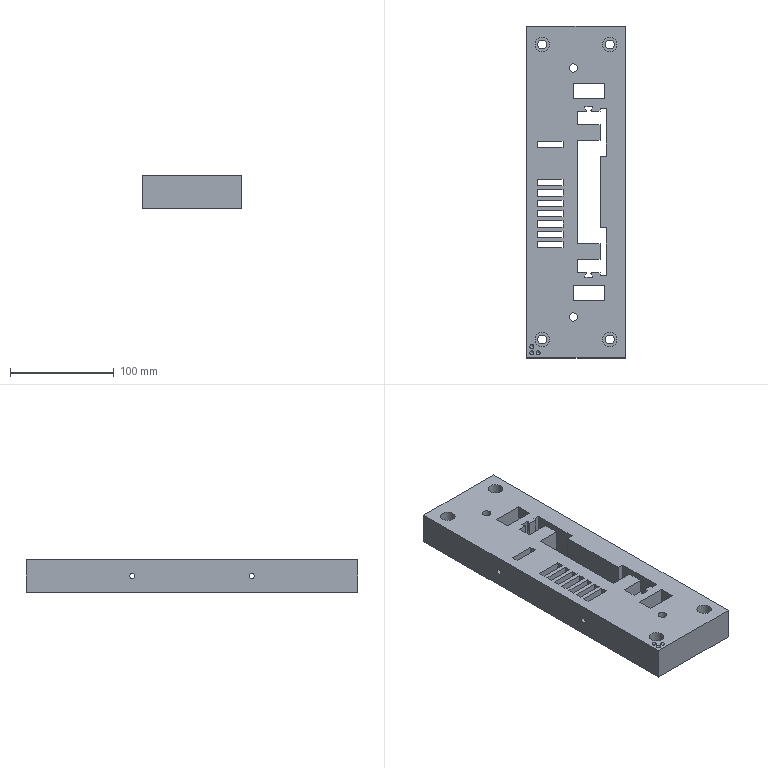Part | STEP file | 200 mesh_id2194 | 1 solid | 109 faces | box 95 x 320 x 31.2 mm | volume 758005 mm3 | plane 78 | cylinder 24 | cone 7 | commonest cylinder face diameters 0.52 x4 1.08 x4 5.02 x4 8.6 x4 14 x4 6.8 x2